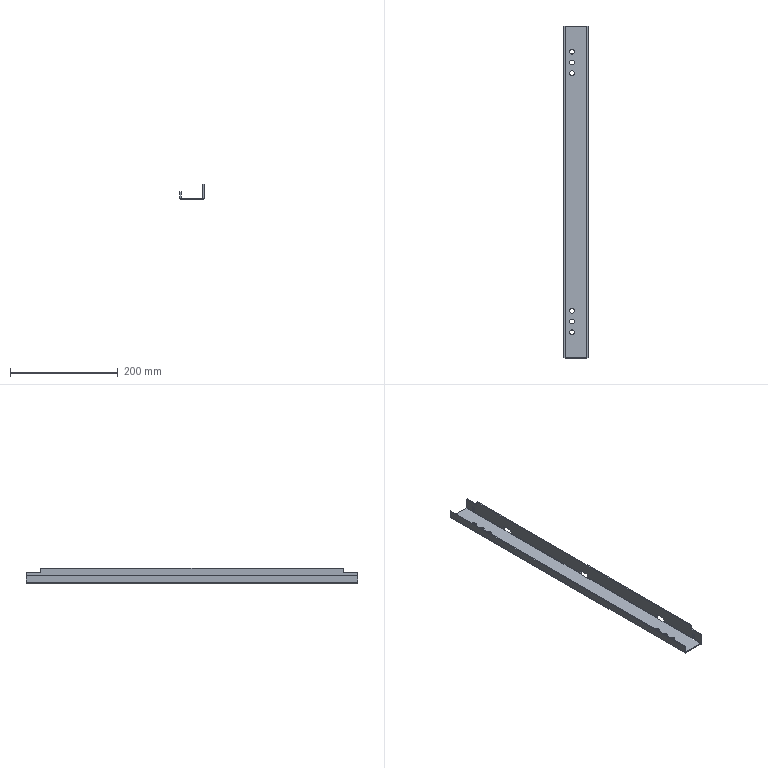Part | STEP file | Instrument door gasket strip vertical (hinge) modified | 1 solid | 88 faces | box 44.5 x 615 x 28.5 mm | volume 98883 mm3 | plane 62 | cylinder 26 | commonest cylinder face diameters 9 x12 1 x7 5 x7